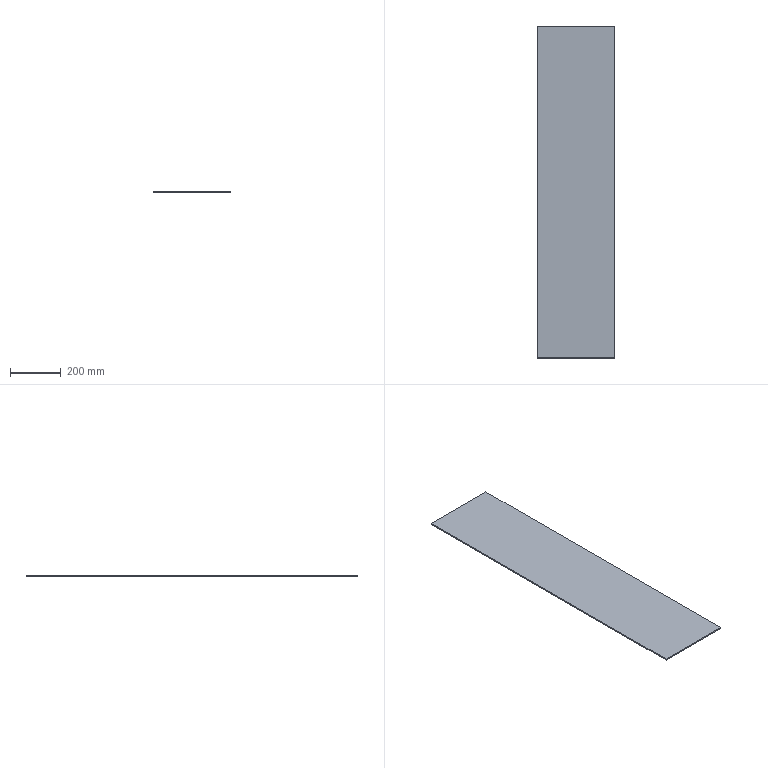Part | SolidWorks | features Extrusion 1, HoleWzd 1 | 1 solid | 6 faces | box 304 x 1306 x 5 mm | volume 1985120 mm3 | plane 6
STEP:
#1=CARTESIAN_POINT('',(152.,-653.,0.));
#2=VERTEX_POINT('',#1);
#3=CARTESIAN_POINT('',(152.,653.,0.));
#4=VERTEX_POINT('',#3);
#5=CARTESIAN_POINT('',(152.,653.,0.));
#6=DIRECTION('',(0.,1.,0.));
#7=VECTOR('',#6,1000.);
#8=LINE('',#5,#7);
#9=EDGE_CURVE('',#2,#4,#8,.T.);
#10=ORIENTED_EDGE('',*,*,#9,.T.);
#11=CARTESIAN_POINT('',(152.,653.,5.));
#12=VERTEX_POINT('',#11);
#13=CARTESIAN_POINT('',(152.,653.,5.));
#14=DIRECTION('',(0.,0.,-1.));
#15=VECTOR('',#14,1000.);
#16=LINE('',#13,#15);
#17=EDGE_CURVE('',#12,#4,#16,.T.);
#18=ORIENTED_EDGE('',*,*,#17,.F.);
#19=CARTESIAN_POINT('',(152.,-653.,5.));
#20=VERTEX_POINT('',#19);
#21=CARTESIAN_POINT('',(152.,653.,5.));
#22=DIRECTION('',(0.,1.,0.));
#23=VECTOR('',#22,1000.);
#24=LINE('',#21,#23);
#25=EDGE_CURVE('',#20,#12,#24,.T.);
#26=ORIENTED_EDGE('',*,*,#25,.F.);
#27=CARTESIAN_POINT('',(152.,-653.,5.));
#28=DIRECTION('',(0.,0.,-1.));
#29=VECTOR('',#28,1000.);
#30=LINE('',#27,#29);
#31=EDGE_CURVE('',#20,#2,#30,.T.);
#32=ORIENTED_EDGE('',*,*,#31,.T.);
#33=EDGE_LOOP('',(#10,#18,#26,#32));
#34=FACE_OUTER_BOUND('',#33,.T.);
#35=CARTESIAN_POINT('',(152.,653.,5.));
#36=DIRECTION('',(-1.,0.,0.));
#37=DIRECTION('',(0.,-1.,0.));
#38=AXIS2_PLACEMENT_3D('',#35,#36,#37);
#39=PLANE('',#38);
#40=ADVANCED_FACE('',(#34),#39,.F.);
#41=CARTESIAN_POINT('',(-152.,653.,0.));
#42=VERTEX_POINT('',#41);
#43=CARTESIAN_POINT('',(-152.,653.,0.));
#44=DIRECTION('',(-1.,0.,0.));
#45=VECTOR('',#44,1000.);
#46=LINE('',#43,#45);
#47=EDGE_CURVE('',#4,#42,#46,.T.);
#48=ORIENTED_EDGE('',*,*,#47,.T.);
#49=CARTESIAN_POINT('',(-152.,653.,5.));
#50=VERTEX_POINT('',#49);
#51=CARTESIAN_POINT('',(-152.,653.,5.));
#52=DIRECTION('',(0.,0.,-1.));
#53=VECTOR('',#52,1000.);
#54=LINE('',#51,#53);
#55=EDGE_CURVE('',#50,#42,#54,.T.);
#56=ORIENTED_EDGE('',*,*,#55,.F.);
#57=CARTESIAN_POINT('',(-152.,653.,5.));
#58=DIRECTION('',(-1.,0.,0.));
#59=VECTOR('',#58,1000.);
#60=LINE('',#57,#59);
#61=EDGE_CURVE('',#12,#50,#60,.T.);
#62=ORIENTED_EDGE('',*,*,#61,.F.);
#63=ORIENTED_EDGE('',*,*,#17,.T.);
#64=EDGE_LOOP('',(#48,#56,#62,#63));
#65=FACE_OUTER_BOUND('',#64,.T.);
#66=CARTESIAN_POINT('',(-152.,653.,5.));
#67=DIRECTION('',(0.,-1.,0.));
#68=DIRECTION('',(0.,0.,-1.));
#69=AXIS2_PLACEMENT_3D('',#66,#67,#68);
#70=PLANE('',#69);
#71=ADVANCED_FACE('',(#65),#70,.F.);
#72=CARTESIAN_POINT('',(-152.,-653.,0.));
#73=VERTEX_POINT('',#72);
#74=CARTESIAN_POINT('',(-152.,653.,0.));
#75=DIRECTION('',(0.,-1.,0.));
#76=VECTOR('',#75,1000.);
#77=LINE('',#74,#76);
#78=EDGE_CURVE('',#42,#73,#77,.T.);
#79=ORIENTED_EDGE('',*,*,#78,.T.);
#80=CARTESIAN_POINT('',(-152.,-653.,5.));
#81=VERTEX_POINT('',#80);
#82=CARTESIAN_POINT('',(-152.,-653.,5.));
#83=DIRECTION('',(0.,0.,-1.));
#84=VECTOR('',#83,1000.);
#85=LINE('',#82,#84);
#86=EDGE_CURVE('',#81,#73,#85,.T.);
#87=ORIENTED_EDGE('',*,*,#86,.F.);
#88=CARTESIAN_POINT('',(-152.,653.,5.));
#89=DIRECTION('',(0.,-1.,0.));
#90=VECTOR('',#89,1000.);
#91=LINE('',#88,#90);
#92=EDGE_CURVE('',#50,#81,#91,.T.);
#93=ORIENTED_EDGE('',*,*,#92,.F.);
#94=ORIENTED_EDGE('',*,*,#55,.T.);
#95=EDGE_LOOP('',(#79,#87,#93,#94));
#96=FACE_OUTER_BOUND('',#95,.T.);
#97=CARTESIAN_POINT('',(-152.,653.,5.));
#98=DIRECTION('',(1.,0.,0.));
#99=DIRECTION('',(0.,1.,0.));
#100=AXIS2_PLACEMENT_3D('',#97,#98,#99);
#101=PLANE('',#100);
#102=ADVANCED_FACE('',(#96),#101,.F.);
#103=CARTESIAN_POINT('',(-152.,-653.,0.));
#104=DIRECTION('',(1.,0.,0.));
#105=VECTOR('',#104,1000.);
#106=LINE('',#103,#105);
#107=EDGE_CURVE('',#73,#2,#106,.T.);
#108=ORIENTED_EDGE('',*,*,#107,.T.);
#109=ORIENTED_EDGE('',*,*,#31,.F.);
#110=CARTESIAN_POINT('',(-152.,-653.,5.));
#111=DIRECTION('',(1.,0.,0.));
#112=VECTOR('',#111,1000.);
#113=LINE('',#110,#112);
#114=EDGE_CURVE('',#81,#20,#113,.T.);
#115=ORIENTED_EDGE('',*,*,#114,.F.);
#116=ORIENTED_EDGE('',*,*,#86,.T.);
#117=EDGE_LOOP('',(#108,#109,#115,#116));
#118=FACE_OUTER_BOUND('',#117,.T.);
#119=CARTESIAN_POINT('',(-152.,-653.,5.));
#120=DIRECTION('',(0.,1.,0.));
#121=DIRECTION('',(0.,0.,1.));
#122=AXIS2_PLACEMENT_3D('',#119,#120,#121);
#123=PLANE('',#122);
#124=ADVANCED_FACE('',(#118),#123,.F.);
#125=ORIENTED_EDGE('',*,*,#25,.T.);
#126=ORIENTED_EDGE('',*,*,#61,.T.);
#127=ORIENTED_EDGE('',*,*,#92,.T.);
#128=ORIENTED_EDGE('',*,*,#114,.T.);
#129=EDGE_LOOP('',(#125,#126,#127,#128));
#130=FACE_OUTER_BOUND('',#129,.T.);
#131=CARTESIAN_POINT('',(0.,0.,5.));
#132=DIRECTION('',(0.,0.,1.));
#133=DIRECTION('',(1.,0.,0.));
#134=AXIS2_PLACEMENT_3D('',#131,#132,#133);
#135=PLANE('',#134);
#136=ADVANCED_FACE('',(#130),#135,.T.);
#137=ORIENTED_EDGE('',*,*,#9,.F.);
#138=ORIENTED_EDGE('',*,*,#107,.F.);
#139=ORIENTED_EDGE('',*,*,#78,.F.);
#140=ORIENTED_EDGE('',*,*,#47,.F.);
#141=EDGE_LOOP('',(#137,#138,#139,#140));
#142=FACE_OUTER_BOUND('',#141,.T.);
#143=CARTESIAN_POINT('',(0.,0.,0.));
#144=DIRECTION('',(0.,0.,1.));
#145=DIRECTION('',(1.,0.,0.));
#146=AXIS2_PLACEMENT_3D('',#143,#144,#145);
#147=PLANE('',#146);
#148=ADVANCED_FACE('',(#142),#147,.F.);
#149=CLOSED_SHELL('',(#40,#71,#102,#124,#136,#148));
#150=MANIFOLD_SOLID_BREP('',#149);
#151=CARTESIAN_POINT('',(0.,0.,0.));
#152=DIRECTION('',(0.,0.,1.));
#153=DIRECTION('',(1.,0.,0.));
#154=AXIS2_PLACEMENT_3D('',#151,#152,#153);
#155=(LENGTH_UNIT()NAMED_UNIT(*)SI_UNIT(.MILLI.,.METRE.));
#156=UNCERTAINTY_MEASURE_WITH_UNIT(LENGTH_MEASURE(0.00001),#155,'','');
#157=(NAMED_UNIT(*)PLANE_ANGLE_UNIT()SI_UNIT($,.RADIAN.));
#158=(NAMED_UNIT(*)SI_UNIT($,.STERADIAN.)SOLID_ANGLE_UNIT());
#159=(GEOMETRIC_REPRESENTATION_CONTEXT(3)GLOBAL_UNCERTAINTY_ASSIGNED_CONTEXT((#156))GLOBAL_UNIT_ASSIGNED_CONTEXT((#155,#157,#158))REPRESENTATION_CONTEXT('',''));
#160=ADVANCED_BREP_SHAPE_REPRESENTATION('',(#150,#154),#159);